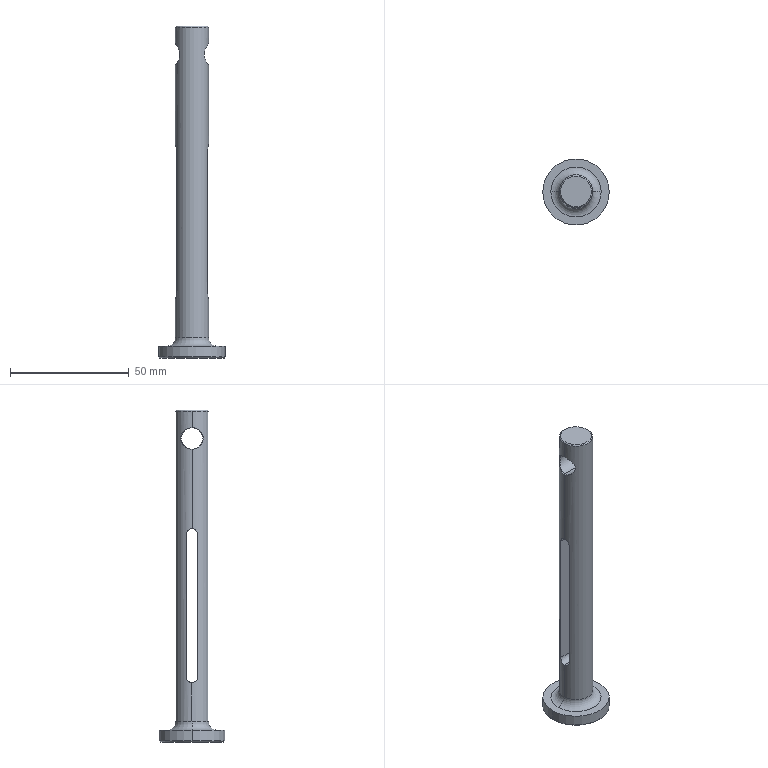Part | SolidWorks | features Chamfer 3, ICE 3, Extrusion 1, Fillet 1 | 1 solid | 24 faces | box 28 x 28 x 140 mm | volume 18757 mm3 | cylinder 9 | plane 5 | spline 4 | cone 4 | torus 2 | commonest cylinder face diameters 5 x3 9 x2 14 x2 28 x2